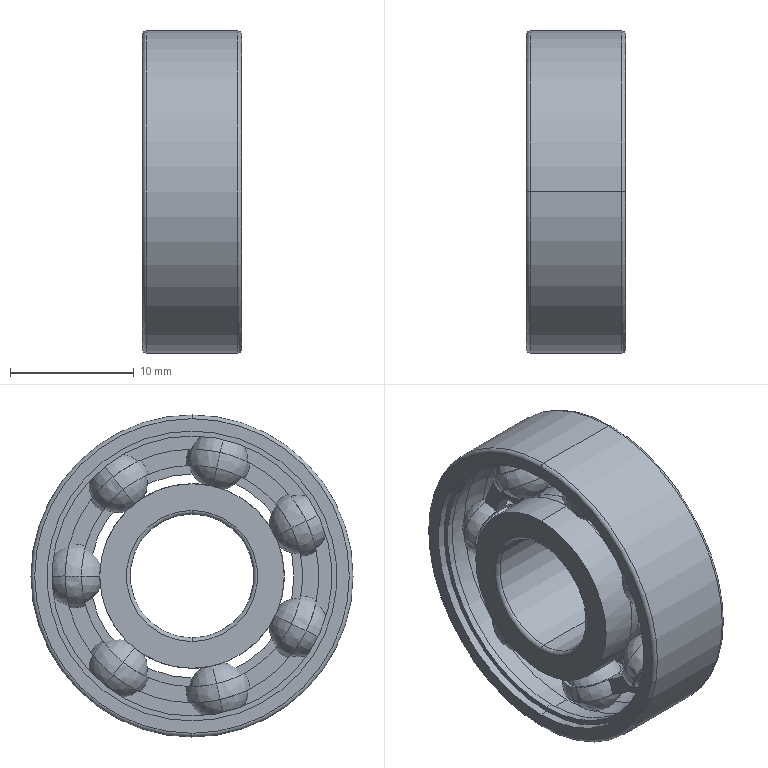Part | NX | features BREP 1 | 1 solid | 134 faces | box 8 x 26 x 26 mm | volume 2122 mm3 | sphere 56 | torus 32 | cylinder 24 | plane 22 | commonest cylinder face diameters 23.4 x8 14.9 x4 10 x2 16.471 x2 17.84 x2 20.46 x2